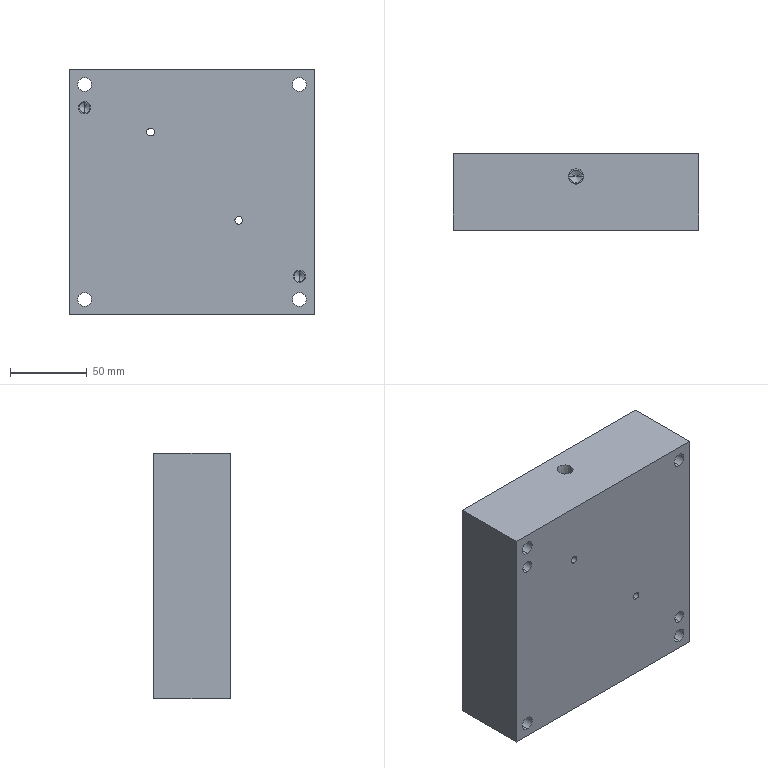Part | STEP file | OP10-109_base block (lower)-R | 1 solid | 112 faces | box 160 x 50 x 160 mm | volume 1246879 mm3 | cylinder 74 | plane 30 | cone 8 | commonest cylinder face diameters 6 x8 9 x8 14 x8 20 x7 25.8 x7 5 x4